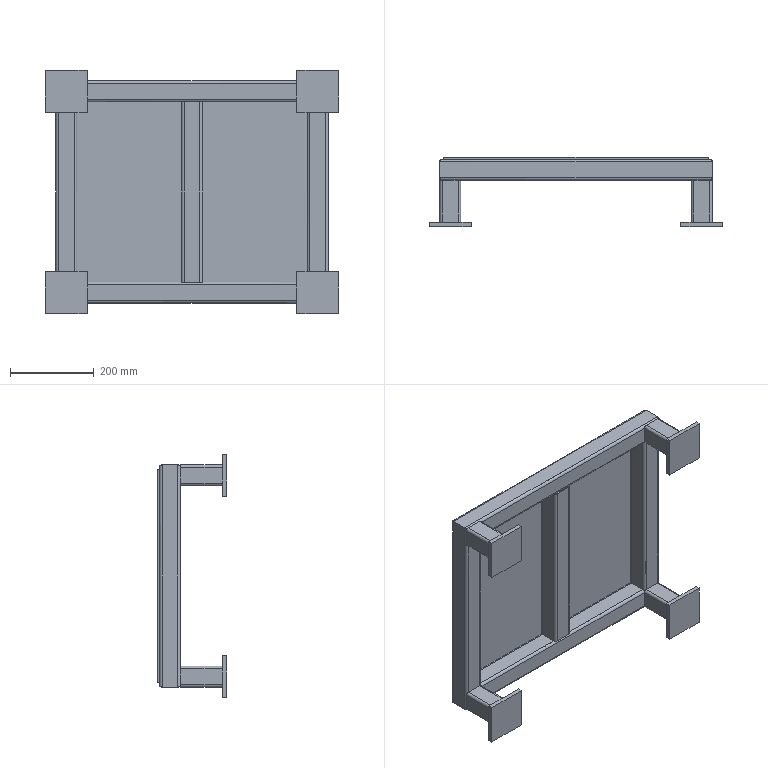Part | STEP file | HXGR200008-07 | 14 solids | 192 faces | box 700 x 165 x 580 mm | volume 3623561 mm3 | plane 120 | cylinder 72 | commonest cylinder face diameters 6 x36 12 x36